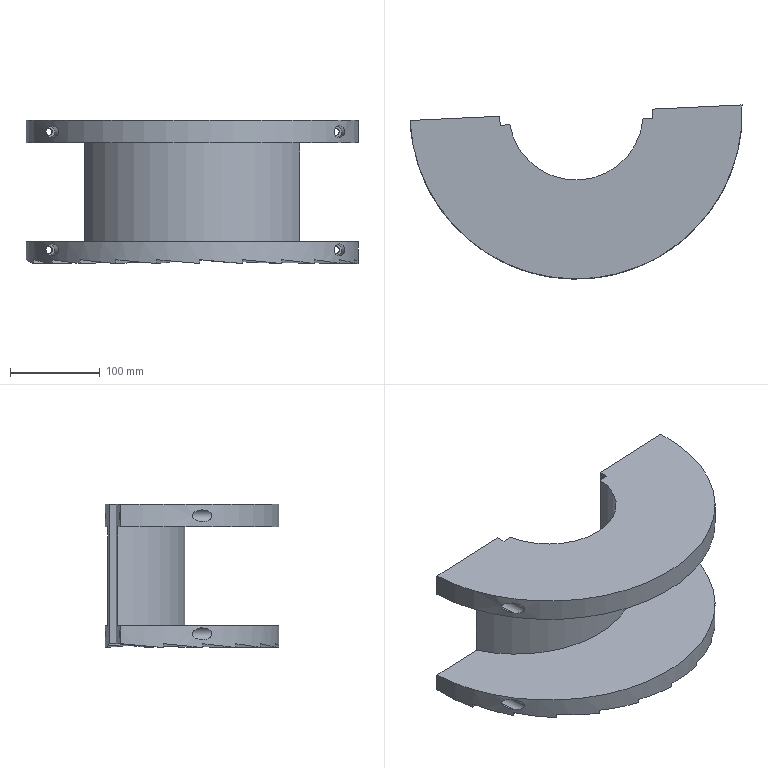Part | SolidWorks | features BaseBody 1 | 1 solid | 69 faces | box 369.799 x 193.623 x 159.255 mm | volume 2559230 mm3 | plane 37 | cylinder 32 | commonest cylinder face diameters 220 x12 8 x8 13 x8 370 x2 150 x1 260 x1